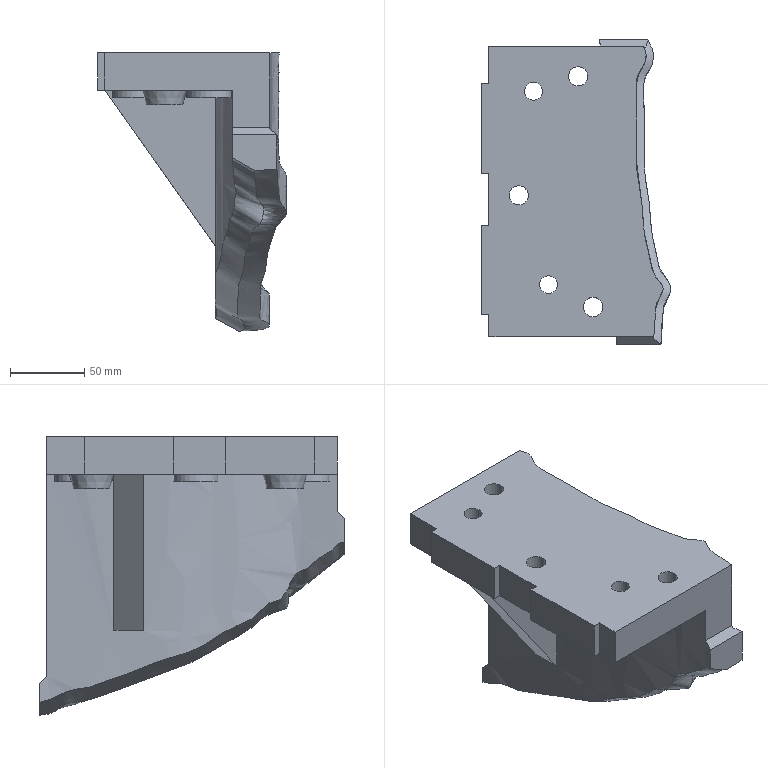Part | NX | features solid 2 | 1 solid | 45 faces | box 127.016 x 205 x 187.055 mm | volume 1206755 mm3 | plane 27 | cylinder 10 | spline 6 | cone 2 | commonest cylinder face diameters 13 x5 30 x3 12 x2